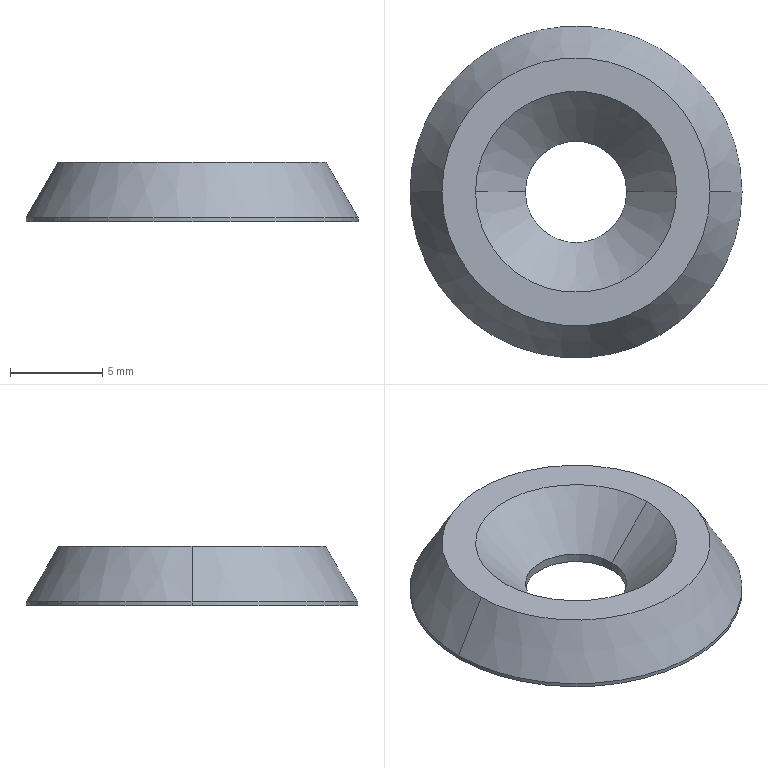Part | STEP file | Stainless steel conical countersunk washer M5 | 1 solid | 10 faces | box 18 x 18 x 3.2 mm | volume 517.188 mm3 | cone 4 | cylinder 4 | plane 2 | commonest cylinder face diameters 5.5 x2 18 x2
STEP:
#1=CARTESIAN_POINT('',(0.,0.,0.));
#2=DIRECTION('',(0.,0.,1.));
#3=DIRECTION('',(1.,0.,0.));
#4=AXIS2_PLACEMENT_3D('',#1,#2,#3);
#5=CARTESIAN_POINT('',(7.268,0.,1.6));
#6=VERTEX_POINT('',#5);
#7=CARTESIAN_POINT('',(-7.268,0.,1.6));
#8=VERTEX_POINT('',#7);
#9=CARTESIAN_POINT('',(0.,0.,1.6));
#10=DIRECTION('',(0.,0.,1.));
#11=DIRECTION('',(1.,0.,0.));
#12=AXIS2_PLACEMENT_3D('',#9,#10,#11);
#13=CIRCLE('',#12,7.268);
#14=CARTESIAN_POINT('',(0.,0.,1.6));
#15=DIRECTION('',(0.,0.,-1.));
#16=DIRECTION('',(-1.,0.,0.));
#17=AXIS2_PLACEMENT_3D('',#14,#15,#16);
#18=CONICAL_SURFACE('',#17,7.268,0.5236);
#19=CARTESIAN_POINT('',(3.142,0.));
#20=DIRECTION('',(-1.,0.));
#21=VECTOR('',#20,1.);
#22=LINE('',#19,#21);
#23=(GEOMETRIC_REPRESENTATION_CONTEXT(2)PARAMETRIC_REPRESENTATION_CONTEXT()REPRESENTATION_CONTEXT('',''));
#24=DEFINITIONAL_REPRESENTATION('',(#22),#23);
#25=PCURVE('',#18,#24);
#26=CARTESIAN_POINT('',(0.,0.,1.6));
#27=DIRECTION('',(0.,0.,1.));
#28=DIRECTION('',(1.,0.,0.));
#29=AXIS2_PLACEMENT_3D('',#26,#27,#28);
#30=PLANE('',#29);
#31=CARTESIAN_POINT('',(0.,0.));
#32=DIRECTION('',(1.,0.));
#33=AXIS2_PLACEMENT_2D('',#31,#32);
#34=CIRCLE('',#33,7.268);
#35=(GEOMETRIC_REPRESENTATION_CONTEXT(2)PARAMETRIC_REPRESENTATION_CONTEXT()REPRESENTATION_CONTEXT('',''));
#36=DEFINITIONAL_REPRESENTATION('',(#34),#35);
#37=PCURVE('',#30,#36);
#38=SURFACE_CURVE('',#13,(#25,#37),.PCURVE_S1.);
#39=EDGE_CURVE('',#6,#8,#38,.T.);
#40=ORIENTED_EDGE('',*,*,#39,.F.);
#41=CARTESIAN_POINT('',(9.,0.,-1.4));
#42=VERTEX_POINT('',#41);
#43=CARTESIAN_POINT('',(7.268,0.,1.6));
#44=DIRECTION('',(0.5,0.,-0.866));
#45=VECTOR('',#44,1.);
#46=LINE('',#43,#45);
#47=CARTESIAN_POINT('',(3.142,0.));
#48=DIRECTION('',(0.,1.));
#49=VECTOR('',#48,1.);
#50=LINE('',#47,#49);
#51=(GEOMETRIC_REPRESENTATION_CONTEXT(2)PARAMETRIC_REPRESENTATION_CONTEXT()REPRESENTATION_CONTEXT('',''));
#52=DEFINITIONAL_REPRESENTATION('',(#50),#51);
#53=PCURVE('',#18,#52);
#54=CARTESIAN_POINT('',(0.,0.,1.6));
#55=DIRECTION('',(0.,0.,-1.));
#56=DIRECTION('',(-1.,0.,0.));
#57=AXIS2_PLACEMENT_3D('',#54,#55,#56);
#58=CONICAL_SURFACE('',#57,7.268,0.5236);
#59=CARTESIAN_POINT('',(3.142,0.));
#60=DIRECTION('',(0.,1.));
#61=VECTOR('',#60,1.);
#62=LINE('',#59,#61);
#63=(GEOMETRIC_REPRESENTATION_CONTEXT(2)PARAMETRIC_REPRESENTATION_CONTEXT()REPRESENTATION_CONTEXT('',''));
#64=DEFINITIONAL_REPRESENTATION('',(#62),#63);
#65=PCURVE('',#58,#64);
#66=SURFACE_CURVE('',#46,(#53,#65),.PCURVE_S1.);
#67=EDGE_CURVE('',#6,#42,#66,.T.);
#68=ORIENTED_EDGE('',*,*,#67,.T.);
#69=CARTESIAN_POINT('',(-9.,0.,-1.4));
#70=VERTEX_POINT('',#69);
#71=CARTESIAN_POINT('',(0.,0.,-1.4));
#72=DIRECTION('',(0.,0.,-1.));
#73=DIRECTION('',(1.,0.,0.));
#74=AXIS2_PLACEMENT_3D('',#71,#72,#73);
#75=CIRCLE('',#74,9.);
#76=CARTESIAN_POINT('',(-3.142,3.));
#77=DIRECTION('',(1.,0.));
#78=VECTOR('',#77,1.);
#79=LINE('',#76,#78);
#80=(GEOMETRIC_REPRESENTATION_CONTEXT(2)PARAMETRIC_REPRESENTATION_CONTEXT()REPRESENTATION_CONTEXT('',''));
#81=DEFINITIONAL_REPRESENTATION('',(#79),#80);
#82=PCURVE('',#18,#81);
#83=CARTESIAN_POINT('',(0.,0.,1.6));
#84=DIRECTION('',(0.,0.,-1.));
#85=DIRECTION('',(-1.,0.,0.));
#86=AXIS2_PLACEMENT_3D('',#83,#84,#85);
#87=CYLINDRICAL_SURFACE('',#86,9.);
#88=CARTESIAN_POINT('',(-3.142,3.));
#89=DIRECTION('',(1.,0.));
#90=VECTOR('',#89,1.);
#91=LINE('',#88,#90);
#92=(GEOMETRIC_REPRESENTATION_CONTEXT(2)PARAMETRIC_REPRESENTATION_CONTEXT()REPRESENTATION_CONTEXT('',''));
#93=DEFINITIONAL_REPRESENTATION('',(#91),#92);
#94=PCURVE('',#87,#93);
#95=SURFACE_CURVE('',#75,(#82,#94),.PCURVE_S1.);
#96=EDGE_CURVE('',#70,#42,#95,.T.);
#97=ORIENTED_EDGE('',*,*,#96,.F.);
#98=CARTESIAN_POINT('',(-7.268,0.,1.6));
#99=DIRECTION('',(-0.5,0.,-0.866));
#100=VECTOR('',#99,1.);
#101=LINE('',#98,#100);
#102=CARTESIAN_POINT('',(0.,0.));
#103=DIRECTION('',(0.,1.));
#104=VECTOR('',#103,1.);
#105=LINE('',#102,#104);
#106=(GEOMETRIC_REPRESENTATION_CONTEXT(2)PARAMETRIC_REPRESENTATION_CONTEXT()REPRESENTATION_CONTEXT('',''));
#107=DEFINITIONAL_REPRESENTATION('',(#105),#106);
#108=PCURVE('',#18,#107);
#109=CARTESIAN_POINT('',(6.283,0.));
#110=DIRECTION('',(0.,1.));
#111=VECTOR('',#110,1.);
#112=LINE('',#109,#111);
#113=(GEOMETRIC_REPRESENTATION_CONTEXT(2)PARAMETRIC_REPRESENTATION_CONTEXT()REPRESENTATION_CONTEXT('',''));
#114=DEFINITIONAL_REPRESENTATION('',(#112),#113);
#115=PCURVE('',#58,#114);
#116=SURFACE_CURVE('',#101,(#108,#115),.PCURVE_S1.);
#117=EDGE_CURVE('',#8,#70,#116,.T.);
#118=ORIENTED_EDGE('',*,*,#117,.F.);
#119=EDGE_LOOP('',(#40,#68,#97,#118));
#120=FACE_BOUND('',#119,.T.);
#121=ADVANCED_FACE('',(#120),#18,.T.);
#122=CARTESIAN_POINT('',(2.75,0.,-1.1));
#123=VERTEX_POINT('',#122);
#124=CARTESIAN_POINT('',(5.45,0.,1.6));
#125=VERTEX_POINT('',#124);
#126=CARTESIAN_POINT('',(2.75,0.,-1.1));
#127=DIRECTION('',(0.7071,0.,0.7071));
#128=VECTOR('',#127,1.);
#129=LINE('',#126,#128);
#130=CARTESIAN_POINT('',(0.,0.,-1.1));
#131=DIRECTION('',(0.,0.,1.));
#132=DIRECTION('',(1.,0.,0.));
#133=AXIS2_PLACEMENT_3D('',#130,#131,#132);
#134=CONICAL_SURFACE('',#133,2.75,0.7854);
#135=CARTESIAN_POINT('',(6.283,0.));
#136=DIRECTION('',(0.,1.));
#137=VECTOR('',#136,1.);
#138=LINE('',#135,#137);
#139=(GEOMETRIC_REPRESENTATION_CONTEXT(2)PARAMETRIC_REPRESENTATION_CONTEXT()REPRESENTATION_CONTEXT('',''));
#140=DEFINITIONAL_REPRESENTATION('',(#138),#139);
#141=PCURVE('',#134,#140);
#142=CARTESIAN_POINT('',(0.,0.,-1.1));
#143=DIRECTION('',(0.,0.,1.));
#144=DIRECTION('',(1.,0.,0.));
#145=AXIS2_PLACEMENT_3D('',#142,#143,#144);
#146=CONICAL_SURFACE('',#145,2.75,0.7854);
#147=CARTESIAN_POINT('',(0.,0.));
#148=DIRECTION('',(0.,1.));
#149=VECTOR('',#148,1.);
#150=LINE('',#147,#149);
#151=(GEOMETRIC_REPRESENTATION_CONTEXT(2)PARAMETRIC_REPRESENTATION_CONTEXT()REPRESENTATION_CONTEXT('',''));
#152=DEFINITIONAL_REPRESENTATION('',(#150),#151);
#153=PCURVE('',#146,#152);
#154=SURFACE_CURVE('',#129,(#141,#153),.PCURVE_S1.);
#155=EDGE_CURVE('',#123,#125,#154,.T.);
#156=ORIENTED_EDGE('',*,*,#155,.T.);
#157=CARTESIAN_POINT('',(-5.45,0.,1.6));
#158=VERTEX_POINT('',#157);
#159=CARTESIAN_POINT('',(0.,0.,1.6));
#160=DIRECTION('',(0.,0.,-1.));
#161=DIRECTION('',(1.,0.,0.));
#162=AXIS2_PLACEMENT_3D('',#159,#160,#161);
#163=CIRCLE('',#162,5.45);
#164=CARTESIAN_POINT('',(6.283,2.7));
#165=DIRECTION('',(-1.,0.));
#166=VECTOR('',#165,1.);
#167=LINE('',#164,#166);
#168=(GEOMETRIC_REPRESENTATION_CONTEXT(2)PARAMETRIC_REPRESENTATION_CONTEXT()REPRESENTATION_CONTEXT('',''));
#169=DEFINITIONAL_REPRESENTATION('',(#167),#168);
#170=PCURVE('',#134,#169);
#171=CARTESIAN_POINT('',(5.45,0.));
#172=CARTESIAN_POINT('',(5.45,-9.44));
#173=CARTESIAN_POINT('',(-2.725,-4.72));
#174=CARTESIAN_POINT('',(-10.9,0.));
#175=CARTESIAN_POINT('',(-2.725,4.72));
#176=CARTESIAN_POINT('',(5.45,9.44));
#177=CARTESIAN_POINT('',(5.45,0.));
#178=(BOUNDED_CURVE()B_SPLINE_CURVE(2,(#171,#172,#173,#174,#175,#176,#177),.UNSPECIFIED.,.T.,.F.)B_SPLINE_CURVE_WITH_KNOTS((1,2,2,2,2,1),(-2.094,0.,2.094,4.189,6.283,8.378),.UNSPECIFIED.)CURVE()GEOMETRIC_REPRESENTATION_ITEM()RATIONAL_B_SPLINE_CURVE((1.,0.5,1.,0.5,1.,0.5,1.))REPRESENTATION_ITEM(''));
#179=(GEOMETRIC_REPRESENTATION_CONTEXT(2)PARAMETRIC_REPRESENTATION_CONTEXT()REPRESENTATION_CONTEXT('',''));
#180=DEFINITIONAL_REPRESENTATION('',(#178),#179);
#181=PCURVE('',#30,#180);
#182=SURFACE_CURVE('',#163,(#170,#181),.PCURVE_S1.);
#183=EDGE_CURVE('',#125,#158,#182,.T.);
#184=ORIENTED_EDGE('',*,*,#183,.T.);
#185=CARTESIAN_POINT('',(-2.75,0.,-1.1));
#186=VERTEX_POINT('',#185);
#187=CARTESIAN_POINT('',(-2.75,0.,-1.1));
#188=DIRECTION('',(-0.7071,0.,0.7071));
#189=VECTOR('',#188,1.);
#190=LINE('',#187,#189);
#191=CARTESIAN_POINT('',(3.142,0.));
#192=DIRECTION('',(0.,1.));
#193=VECTOR('',#192,1.);
#194=LINE('',#191,#193);
#195=(GEOMETRIC_REPRESENTATION_CONTEXT(2)PARAMETRIC_REPRESENTATION_CONTEXT()REPRESENTATION_CONTEXT('',''));
#196=DEFINITIONAL_REPRESENTATION('',(#194),#195);
#197=PCURVE('',#134,#196);
#198=CARTESIAN_POINT('',(3.142,0.));
#199=DIRECTION('',(0.,1.));
#200=VECTOR('',#199,1.);
#201=LINE('',#198,#200);
#202=(GEOMETRIC_REPRESENTATION_CONTEXT(2)PARAMETRIC_REPRESENTATION_CONTEXT()REPRESENTATION_CONTEXT('',''));
#203=DEFINITIONAL_REPRESENTATION('',(#201),#202);
#204=PCURVE('',#146,#203);
#205=SURFACE_CURVE('',#190,(#197,#204),.PCURVE_S1.);
#206=EDGE_CURVE('',#186,#158,#205,.T.);
#207=ORIENTED_EDGE('',*,*,#206,.F.);
#208=CARTESIAN_POINT('',(0.,0.,-1.1));
#209=DIRECTION('',(0.,0.,1.));
#210=DIRECTION('',(1.,0.,0.));
#211=AXIS2_PLACEMENT_3D('',#208,#209,#210);
#212=CIRCLE('',#211,2.75);
#213=CARTESIAN_POINT('',(0.,0.));
#214=DIRECTION('',(1.,0.));
#215=VECTOR('',#214,1.);
#216=LINE('',#213,#215);
#217=(GEOMETRIC_REPRESENTATION_CONTEXT(2)PARAMETRIC_REPRESENTATION_CONTEXT()REPRESENTATION_CONTEXT('',''));
#218=DEFINITIONAL_REPRESENTATION('',(#216),#217);
#219=PCURVE('',#134,#218);
#220=CARTESIAN_POINT('',(0.,0.,1.6));
#221=DIRECTION('',(0.,0.,-1.));
#222=DIRECTION('',(-1.,0.,0.));
#223=AXIS2_PLACEMENT_3D('',#220,#221,#222);
#224=CYLINDRICAL_SURFACE('',#223,2.75);
#225=CARTESIAN_POINT('',(9.425,2.7));
#226=DIRECTION('',(-1.,0.));
#227=VECTOR('',#226,1.);
#228=LINE('',#225,#227);
#229=(GEOMETRIC_REPRESENTATION_CONTEXT(2)PARAMETRIC_REPRESENTATION_CONTEXT()REPRESENTATION_CONTEXT('',''));
#230=DEFINITIONAL_REPRESENTATION('',(#228),#229);
#231=PCURVE('',#224,#230);
#232=SURFACE_CURVE('',#212,(#219,#231),.PCURVE_S1.);
#233=EDGE_CURVE('',#186,#123,#232,.T.);
#234=ORIENTED_EDGE('',*,*,#233,.T.);
#235=EDGE_LOOP('',(#156,#184,#207,#234));
#236=FACE_BOUND('',#235,.F.);
#237=ADVANCED_FACE('',(#236),#134,.F.);
#238=CARTESIAN_POINT('',(-2.75,0.,-1.6));
#239=VERTEX_POINT('',#238);
#240=CARTESIAN_POINT('',(-2.75,0.,1.6));
#241=DIRECTION('',(0.,0.,-1.));
#242=VECTOR('',#241,1.);
#243=LINE('',#240,#242);
#244=CARTESIAN_POINT('',(6.283,0.));
#245=DIRECTION('',(0.,1.));
#246=VECTOR('',#245,1.);
#247=LINE('',#244,#246);
#248=(GEOMETRIC_REPRESENTATION_CONTEXT(2)PARAMETRIC_REPRESENTATION_CONTEXT()REPRESENTATION_CONTEXT('',''));
#249=DEFINITIONAL_REPRESENTATION('',(#247),#248);
#250=PCURVE('',#224,#249);
#251=CARTESIAN_POINT('',(0.,0.,1.6));
#252=DIRECTION('',(0.,0.,-1.));
#253=DIRECTION('',(-1.,0.,0.));
#254=AXIS2_PLACEMENT_3D('',#251,#252,#253);
#255=CYLINDRICAL_SURFACE('',#254,2.75);
#256=CARTESIAN_POINT('',(0.,0.));
#257=DIRECTION('',(0.,1.));
#258=VECTOR('',#257,1.);
#259=LINE('',#256,#258);
#260=(GEOMETRIC_REPRESENTATION_CONTEXT(2)PARAMETRIC_REPRESENTATION_CONTEXT()REPRESENTATION_CONTEXT('',''));
#261=DEFINITIONAL_REPRESENTATION('',(#259),#260);
#262=PCURVE('',#255,#261);
#263=SURFACE_CURVE('',#243,(#250,#262),.PCURVE_S1.);
#264=EDGE_CURVE('',#186,#239,#263,.T.);
#265=ORIENTED_EDGE('',*,*,#264,.T.);
#266=CARTESIAN_POINT('',(2.75,0.,-1.6));
#267=VERTEX_POINT('',#266);
#268=CARTESIAN_POINT('',(0.,0.,-1.6));
#269=DIRECTION('',(0.,0.,1.));
#270=DIRECTION('',(1.,0.,0.));
#271=AXIS2_PLACEMENT_3D('',#268,#269,#270);
#272=CIRCLE('',#271,2.75);
#273=CARTESIAN_POINT('',(9.425,3.2));
#274=DIRECTION('',(-1.,0.));
#275=VECTOR('',#274,1.);
#276=LINE('',#273,#275);
#277=(GEOMETRIC_REPRESENTATION_CONTEXT(2)PARAMETRIC_REPRESENTATION_CONTEXT()REPRESENTATION_CONTEXT('',''));
#278=DEFINITIONAL_REPRESENTATION('',(#276),#277);
#279=PCURVE('',#224,#278);
#280=CARTESIAN_POINT('',(0.,0.,-1.6));
#281=DIRECTION('',(0.,0.,1.));
#282=DIRECTION('',(1.,0.,0.));
#283=AXIS2_PLACEMENT_3D('',#280,#281,#282);
#284=PLANE('',#283);
#285=CARTESIAN_POINT('',(0.,0.));
#286=DIRECTION('',(1.,0.));
#287=AXIS2_PLACEMENT_2D('',#285,#286);
#288=CIRCLE('',#287,2.75);
#289=(GEOMETRIC_REPRESENTATION_CONTEXT(2)PARAMETRIC_REPRESENTATION_CONTEXT()REPRESENTATION_CONTEXT('',''));
#290=DEFINITIONAL_REPRESENTATION('',(#288),#289);
#291=PCURVE('',#284,#290);
#292=SURFACE_CURVE('',#272,(#279,#291),.PCURVE_S1.);
#293=EDGE_CURVE('',#239,#267,#292,.T.);
#294=ORIENTED_EDGE('',*,*,#293,.T.);
#295=CARTESIAN_POINT('',(2.75,0.,1.6));
#296=DIRECTION('',(0.,0.,-1.));
#297=VECTOR('',#296,1.);
#298=LINE('',#295,#297);
#299=CARTESIAN_POINT('',(3.142,0.));
#300=DIRECTION('',(0.,1.));
#301=VECTOR('',#300,1.);
#302=LINE('',#299,#301);
#303=(GEOMETRIC_REPRESENTATION_CONTEXT(2)PARAMETRIC_REPRESENTATION_CONTEXT()REPRESENTATION_CONTEXT('',''));
#304=DEFINITIONAL_REPRESENTATION('',(#302),#303);
#305=PCURVE('',#224,#304);
#306=CARTESIAN_POINT('',(3.142,0.));
#307=DIRECTION('',(0.,1.));
#308=VECTOR('',#307,1.);
#309=LINE('',#306,#308);
#310=(GEOMETRIC_REPRESENTATION_CONTEXT(2)PARAMETRIC_REPRESENTATION_CONTEXT()REPRESENTATION_CONTEXT('',''));
#311=DEFINITIONAL_REPRESENTATION('',(#309),#310);
#312=PCURVE('',#255,#311);
#313=SURFACE_CURVE('',#298,(#305,#312),.PCURVE_S1.);
#314=EDGE_CURVE('',#123,#267,#313,.T.);
#315=ORIENTED_EDGE('',*,*,#314,.F.);
#316=ORIENTED_EDGE('',*,*,#233,.F.);
#317=EDGE_LOOP('',(#265,#294,#315,#316));
#318=FACE_BOUND('',#317,.F.);
#319=ADVANCED_FACE('',(#318),#224,.F.);
#320=ORIENTED_EDGE('',*,*,#96,.T.);
#321=CARTESIAN_POINT('',(9.,0.,-1.6));
#322=VERTEX_POINT('',#321);
#323=CARTESIAN_POINT('',(9.,0.,1.6));
#324=DIRECTION('',(0.,0.,-1.));
#325=VECTOR('',#324,1.);
#326=LINE('',#323,#325);
#327=CARTESIAN_POINT('',(3.142,0.));
#328=DIRECTION('',(0.,1.));
#329=VECTOR('',#328,1.);
#330=LINE('',#327,#329);
#331=(GEOMETRIC_REPRESENTATION_CONTEXT(2)PARAMETRIC_REPRESENTATION_CONTEXT()REPRESENTATION_CONTEXT('',''));
#332=DEFINITIONAL_REPRESENTATION('',(#330),#331);
#333=PCURVE('',#87,#332);
#334=CARTESIAN_POINT('',(0.,0.,1.6));
#335=DIRECTION('',(0.,0.,-1.));
#336=DIRECTION('',(-1.,0.,0.));
#337=AXIS2_PLACEMENT_3D('',#334,#335,#336);
#338=CYLINDRICAL_SURFACE('',#337,9.);
#339=CARTESIAN_POINT('',(3.142,0.));
#340=DIRECTION('',(0.,1.));
#341=VECTOR('',#340,1.);
#342=LINE('',#339,#341);
#343=(GEOMETRIC_REPRESENTATION_CONTEXT(2)PARAMETRIC_REPRESENTATION_CONTEXT()REPRESENTATION_CONTEXT('',''));
#344=DEFINITIONAL_REPRESENTATION('',(#342),#343);
#345=PCURVE('',#338,#344);
#346=SURFACE_CURVE('',#326,(#333,#345),.PCURVE_S1.);
#347=EDGE_CURVE('',#42,#322,#346,.T.);
#348=ORIENTED_EDGE('',*,*,#347,.T.);
#349=CARTESIAN_POINT('',(-9.,0.,-1.6));
#350=VERTEX_POINT('',#349);
#351=CARTESIAN_POINT('',(0.,0.,-1.6));
#352=DIRECTION('',(0.,0.,1.));
#353=DIRECTION('',(1.,0.,0.));
#354=AXIS2_PLACEMENT_3D('',#351,#352,#353);
#355=CIRCLE('',#354,9.);
#356=CARTESIAN_POINT('',(3.142,3.2));
#357=DIRECTION('',(-1.,0.));
#358=VECTOR('',#357,1.);
#359=LINE('',#356,#358);
#360=(GEOMETRIC_REPRESENTATION_CONTEXT(2)PARAMETRIC_REPRESENTATION_CONTEXT()REPRESENTATION_CONTEXT('',''));
#361=DEFINITIONAL_REPRESENTATION('',(#359),#360);
#362=PCURVE('',#87,#361);
#363=CARTESIAN_POINT('',(0.,0.));
#364=DIRECTION('',(1.,0.));
#365=AXIS2_PLACEMENT_2D('',#363,#364);
#366=CIRCLE('',#365,9.);
#367=(GEOMETRIC_REPRESENTATION_CONTEXT(2)PARAMETRIC_REPRESENTATION_CONTEXT()REPRESENTATION_CONTEXT('',''));
#368=DEFINITIONAL_REPRESENTATION('',(#366),#367);
#369=PCURVE('',#284,#368);
#370=SURFACE_CURVE('',#355,(#362,#369),.PCURVE_S1.);
#371=EDGE_CURVE('',#322,#350,#370,.T.);
#372=ORIENTED_EDGE('',*,*,#371,.T.);
#373=CARTESIAN_POINT('',(-9.,0.,1.6));
#374=DIRECTION('',(0.,0.,-1.));
#375=VECTOR('',#374,1.);
#376=LINE('',#373,#375);
#377=CARTESIAN_POINT('',(0.,0.));
#378=DIRECTION('',(0.,1.));
#379=VECTOR('',#378,1.);
#380=LINE('',#377,#379);
#381=(GEOMETRIC_REPRESENTATION_CONTEXT(2)PARAMETRIC_REPRESENTATION_CONTEXT()REPRESENTATION_CONTEXT('',''));
#382=DEFINITIONAL_REPRESENTATION('',(#380),#381);
#383=PCURVE('',#87,#382);
#384=CARTESIAN_POINT('',(6.283,0.));
#385=DIRECTION('',(0.,1.));
#386=VECTOR('',#385,1.);
#387=LINE('',#384,#386);
#388=(GEOMETRIC_REPRESENTATION_CONTEXT(2)PARAMETRIC_REPRESENTATION_CONTEXT()REPRESENTATION_CONTEXT('',''));
#389=DEFINITIONAL_REPRESENTATION('',(#387),#388);
#390=PCURVE('',#338,#389);
#391=SURFACE_CURVE('',#376,(#383,#390),.PCURVE_S1.);
#392=EDGE_CURVE('',#70,#350,#391,.T.);
#393=ORIENTED_EDGE('',*,*,#392,.F.);
#394=EDGE_LOOP('',(#320,#348,#372,#393));
#395=FACE_BOUND('',#394,.T.);
#396=ADVANCED_FACE('',(#395),#87,.T.);
#397=CARTESIAN_POINT('',(0.,0.,1.6));
#398=DIRECTION('',(0.,0.,1.));
#399=DIRECTION('',(1.,0.,0.));
#400=AXIS2_PLACEMENT_3D('',#397,#398,#399);
#401=CIRCLE('',#400,7.268);
#402=CARTESIAN_POINT('',(0.,0.));
#403=DIRECTION('',(1.,0.));
#404=AXIS2_PLACEMENT_2D('',#402,#403);
#405=CIRCLE('',#404,7.268);
#406=(GEOMETRIC_REPRESENTATION_CONTEXT(2)PARAMETRIC_REPRESENTATION_CONTEXT()REPRESENTATION_CONTEXT('',''));
#407=DEFINITIONAL_REPRESENTATION('',(#405),#406);
#408=PCURVE('',#30,#407);
#409=CARTESIAN_POINT('',(9.425,0.));
#410=DIRECTION('',(-1.,0.));
#411=VECTOR('',#410,1.);
#412=LINE('',#409,#411);
#413=(GEOMETRIC_REPRESENTATION_CONTEXT(2)PARAMETRIC_REPRESENTATION_CONTEXT()REPRESENTATION_CONTEXT('',''));
#414=DEFINITIONAL_REPRESENTATION('',(#412),#413);
#415=PCURVE('',#58,#414);
#416=SURFACE_CURVE('',#401,(#408,#415),.PCURVE_S1.);
#417=EDGE_CURVE('',#8,#6,#416,.T.);
#418=ORIENTED_EDGE('',*,*,#417,.T.);
#419=ORIENTED_EDGE('',*,*,#39,.T.);
#420=EDGE_LOOP('',(#418,#419));
#421=FACE_BOUND('',#420,.T.);
#422=ORIENTED_EDGE('',*,*,#183,.T.);
#423=CARTESIAN_POINT('',(0.,0.,1.6));
#424=DIRECTION('',(0.,0.,-1.));
#425=DIRECTION('',(1.,0.,0.));
#426=AXIS2_PLACEMENT_3D('',#423,#424,#425);
#427=CIRCLE('',#426,5.45);
#428=CARTESIAN_POINT('',(5.45,0.));
#429=CARTESIAN_POINT('',(5.45,-9.44));
#430=CARTESIAN_POINT('',(-2.725,-4.72));
#431=CARTESIAN_POINT('',(-10.9,0.));
#432=CARTESIAN_POINT('',(-2.725,4.72));
#433=CARTESIAN_POINT('',(5.45,9.44));
#434=CARTESIAN_POINT('',(5.45,0.));
#435=(BOUNDED_CURVE()B_SPLINE_CURVE(2,(#428,#429,#430,#431,#432,#433,#434),.UNSPECIFIED.,.T.,.F.)B_SPLINE_CURVE_WITH_KNOTS((1,2,2,2,2,1),(-2.094,0.,2.094,4.189,6.283,8.378),.UNSPECIFIED.)CURVE()GEOMETRIC_REPRESENTATION_ITEM()RATIONAL_B_SPLINE_CURVE((1.,0.5,1.,0.5,1.,0.5,1.))REPRESENTATION_ITEM(''));
#436=(GEOMETRIC_REPRESENTATION_CONTEXT(2)PARAMETRIC_REPRESENTATION_CONTEXT()REPRESENTATION_CONTEXT('',''));
#437=DEFINITIONAL_REPRESENTATION('',(#435),#436);
#438=PCURVE('',#30,#437);
#439=CARTESIAN_POINT('',(6.283,2.7));
#440=DIRECTION('',(-1.,0.));
#441=VECTOR('',#440,1.);
#442=LINE('',#439,#441);
#443=(GEOMETRIC_REPRESENTATION_CONTEXT(2)PARAMETRIC_REPRESENTATION_CONTEXT()REPRESENTATION_CONTEXT('',''));
#444=DEFINITIONAL_REPRESENTATION('',(#442),#443);
#445=PCURVE('',#146,#444);
#446=SURFACE_CURVE('',#427,(#438,#445),.PCURVE_S1.);
#447=EDGE_CURVE('',#158,#125,#446,.T.);
#448=ORIENTED_EDGE('',*,*,#447,.T.);
#449=EDGE_LOOP('',(#422,#448));
#450=FACE_BOUND('',#449,.T.);
#451=ADVANCED_FACE('',(#421,#450),#30,.T.);
#452=CARTESIAN_POINT('',(0.,0.,-1.6));
#453=DIRECTION('',(0.,0.,1.));
#454=DIRECTION('',(1.,0.,0.));
#455=AXIS2_PLACEMENT_3D('',#452,#453,#454);
#456=CIRCLE('',#455,9.);
#457=CARTESIAN_POINT('',(0.,0.));
#458=DIRECTION('',(1.,0.));
#459=AXIS2_PLACEMENT_2D('',#457,#458);
#460=CIRCLE('',#459,9.);
#461=(GEOMETRIC_REPRESENTATION_CONTEXT(2)PARAMETRIC_REPRESENTATION_CONTEXT()REPRESENTATION_CONTEXT('',''));
#462=DEFINITIONAL_REPRESENTATION('',(#460),#461);
#463=PCURVE('',#284,#462);
#464=CARTESIAN_POINT('',(9.425,3.2));
#465=DIRECTION('',(-1.,0.));
#466=VECTOR('',#465,1.);
#467=LINE('',#464,#466);
#468=(GEOMETRIC_REPRESENTATION_CONTEXT(2)PARAMETRIC_REPRESENTATION_CONTEXT()REPRESENTATION_CONTEXT('',''));
#469=DEFINITIONAL_REPRESENTATION('',(#467),#468);
#470=PCURVE('',#338,#469);
#471=SURFACE_CURVE('',#456,(#463,#470),.PCURVE_S1.);
#472=EDGE_CURVE('',#350,#322,#471,.T.);
#473=ORIENTED_EDGE('',*,*,#472,.F.);
#474=ORIENTED_EDGE('',*,*,#371,.F.);
#475=EDGE_LOOP('',(#473,#474));
#476=FACE_BOUND('',#475,.T.);
#477=ORIENTED_EDGE('',*,*,#293,.T.);
#478=CARTESIAN_POINT('',(0.,0.,-1.6));
#479=DIRECTION('',(0.,0.,1.));
#480=DIRECTION('',(1.,0.,0.));
#481=AXIS2_PLACEMENT_3D('',#478,#479,#480);
#482=CIRCLE('',#481,2.75);
#483=CARTESIAN_POINT('',(0.,0.));
#484=DIRECTION('',(1.,0.));
#485=AXIS2_PLACEMENT_2D('',#483,#484);
#486=CIRCLE('',#485,2.75);
#487=(GEOMETRIC_REPRESENTATION_CONTEXT(2)PARAMETRIC_REPRESENTATION_CONTEXT()REPRESENTATION_CONTEXT('',''));
#488=DEFINITIONAL_REPRESENTATION('',(#486),#487);
#489=PCURVE('',#284,#488);
#490=CARTESIAN_POINT('',(3.142,3.2));
#491=DIRECTION('',(-1.,0.));
#492=VECTOR('',#491,1.);
#493=LINE('',#490,#492);
#494=(GEOMETRIC_REPRESENTATION_CONTEXT(2)PARAMETRIC_REPRESENTATION_CONTEXT()REPRESENTATION_CONTEXT('',''));
#495=DEFINITIONAL_REPRESENTATION('',(#493),#494);
#496=PCURVE('',#255,#495);
#497=SURFACE_CURVE('',#482,(#489,#496),.PCURVE_S1.);
#498=EDGE_CURVE('',#267,#239,#497,.T.);
#499=ORIENTED_EDGE('',*,*,#498,.T.);
#500=EDGE_LOOP('',(#477,#499));
#501=FACE_BOUND('',#500,.T.);
#502=ADVANCED_FACE('',(#476,#501),#284,.F.);
#503=ORIENTED_EDGE('',*,*,#347,.F.);
#504=CARTESIAN_POINT('',(0.,0.,-1.4));
#505=DIRECTION('',(0.,0.,-1.));
#506=DIRECTION('',(1.,0.,0.));
#507=AXIS2_PLACEMENT_3D('',#504,#505,#506);
#508=CIRCLE('',#507,9.);
#509=CARTESIAN_POINT('',(3.142,3.));
#510=DIRECTION('',(1.,0.));
#511=VECTOR('',#510,1.);
#512=LINE('',#509,#511);
#513=(GEOMETRIC_REPRESENTATION_CONTEXT(2)PARAMETRIC_REPRESENTATION_CONTEXT()REPRESENTATION_CONTEXT('',''));
#514=DEFINITIONAL_REPRESENTATION('',(#512),#513);
#515=PCURVE('',#338,#514);
#516=CARTESIAN_POINT('',(3.142,3.));
#517=DIRECTION('',(1.,0.));
#518=VECTOR('',#517,1.);
#519=LINE('',#516,#518);
#520=(GEOMETRIC_REPRESENTATION_CONTEXT(2)PARAMETRIC_REPRESENTATION_CONTEXT()REPRESENTATION_CONTEXT('',''));
#521=DEFINITIONAL_REPRESENTATION('',(#519),#520);
#522=PCURVE('',#58,#521);
#523=SURFACE_CURVE('',#508,(#515,#522),.PCURVE_S1.);
#524=EDGE_CURVE('',#42,#70,#523,.T.);
#525=ORIENTED_EDGE('',*,*,#524,.T.);
#526=ORIENTED_EDGE('',*,*,#392,.T.);
#527=ORIENTED_EDGE('',*,*,#472,.T.);
#528=EDGE_LOOP('',(#503,#525,#526,#527));
#529=FACE_BOUND('',#528,.T.);
#530=ADVANCED_FACE('',(#529),#338,.T.);
#531=ORIENTED_EDGE('',*,*,#498,.T.);
#532=ORIENTED_EDGE('',*,*,#264,.F.);
#533=CARTESIAN_POINT('',(0.,0.,-1.1));
#534=DIRECTION('',(0.,0.,1.));
#535=DIRECTION('',(1.,0.,0.));
#536=AXIS2_PLACEMENT_3D('',#533,#534,#535);
#537=CIRCLE('',#536,2.75);
#538=CARTESIAN_POINT('',(3.142,2.7));
#539=DIRECTION('',(-1.,0.));
#540=VECTOR('',#539,1.);
#541=LINE('',#538,#540);
#542=(GEOMETRIC_REPRESENTATION_CONTEXT(2)PARAMETRIC_REPRESENTATION_CONTEXT()REPRESENTATION_CONTEXT('',''));
#543=DEFINITIONAL_REPRESENTATION('',(#541),#542);
#544=PCURVE('',#255,#543);
#545=CARTESIAN_POINT('',(0.,0.));
#546=DIRECTION('',(1.,0.));
#547=VECTOR('',#546,1.);
#548=LINE('',#545,#547);
#549=(GEOMETRIC_REPRESENTATION_CONTEXT(2)PARAMETRIC_REPRESENTATION_CONTEXT()REPRESENTATION_CONTEXT('',''));
#550=DEFINITIONAL_REPRESENTATION('',(#548),#549);
#551=PCURVE('',#146,#550);
#552=SURFACE_CURVE('',#537,(#544,#551),.PCURVE_S1.);
#553=EDGE_CURVE('',#123,#186,#552,.T.);
#554=ORIENTED_EDGE('',*,*,#553,.F.);
#555=ORIENTED_EDGE('',*,*,#314,.T.);
#556=EDGE_LOOP('',(#531,#532,#554,#555));
#557=FACE_BOUND('',#556,.F.);
#558=ADVANCED_FACE('',(#557),#255,.F.);
#559=ORIENTED_EDGE('',*,*,#447,.T.);
#560=ORIENTED_EDGE('',*,*,#155,.F.);
#561=ORIENTED_EDGE('',*,*,#553,.T.);
#562=ORIENTED_EDGE('',*,*,#206,.T.);
#563=EDGE_LOOP('',(#559,#560,#561,#562));
#564=FACE_BOUND('',#563,.F.);
#565=ADVANCED_FACE('',(#564),#146,.F.);
#566=ORIENTED_EDGE('',*,*,#67,.F.);
#567=ORIENTED_EDGE('',*,*,#417,.F.);
#568=ORIENTED_EDGE('',*,*,#117,.T.);
#569=ORIENTED_EDGE('',*,*,#524,.F.);
#570=EDGE_LOOP('',(#566,#567,#568,#569));
#571=FACE_BOUND('',#570,.T.);
#572=ADVANCED_FACE('',(#571),#58,.T.);
#573=CLOSED_SHELL('',(#121,#237,#319,#396,#451,#502,#530,#558,#565,#572));
#574=MANIFOLD_SOLID_BREP('',#573);
#575=(LENGTH_UNIT()NAMED_UNIT(*)SI_UNIT(.MILLI.,.METRE.));
#576=UNCERTAINTY_MEASURE_WITH_UNIT(LENGTH_MEASURE(0.0000001),#575,'','');
#577=(NAMED_UNIT(*)PLANE_ANGLE_UNIT()SI_UNIT($,.RADIAN.));
#578=(NAMED_UNIT(*)SI_UNIT($,.STERADIAN.)SOLID_ANGLE_UNIT());
#579=(GEOMETRIC_REPRESENTATION_CONTEXT(3)GLOBAL_UNCERTAINTY_ASSIGNED_CONTEXT((#576))GLOBAL_UNIT_ASSIGNED_CONTEXT((#575,#577,#578))REPRESENTATION_CONTEXT('',''));
#580=ADVANCED_BREP_SHAPE_REPRESENTATION('',(#4,#574),#579);